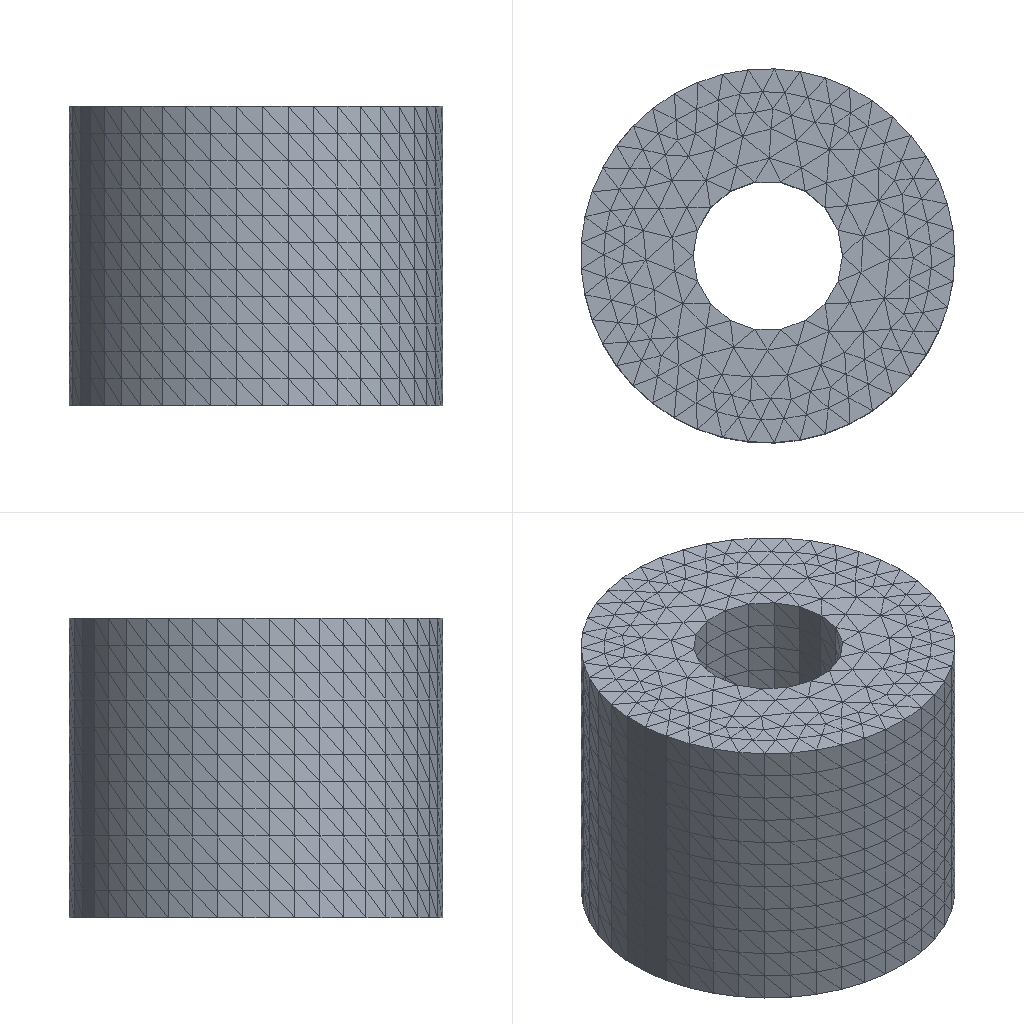Simulation study | abaqus
Notes in the study folder:
10 truncated cone proxy hollow cyl
job_status=None
Umax_mm=0.000227654
S_Mises_max_MPa=1.64312
Set-up summary:
category,name,step,type,value,unit,region
solver,abaqus,,Abaqus/CAE 2024
units,mm-N-s-tonne (MPa),,inferred,E=210000 density=7.85e-09
analysis,Step-1,,static,time_period=1
mesh,nodes,,,14772
mesh,elements,,,9526
element_type,C3D10,,,9526
material,Steel,,E,210000
material,Steel,,nu,0.3
material,Steel,,density,7.85e-09
section,Steel,,solid section,,,_PickedSet2
load,Load,Step-1,pressure,1.2,,TOP
bc,BC,Step-1,encastre,[dofs=ENCASTRE],,FIXED
Abaqus input file, long lists of numbers shortened:
*Heading
** Job name: deck Model name: M10
** Generated by: Abaqus/CAE 2024
*Preprint, echo=NO, model=NO, history=NO, contact=NO
**
** PARTS
**
*Part, name=P
*Node
      1,          10.,           0.,          40.
      2,          10.,           0.,           0.
** (14770 more lines like these left out)
*Element, type=C3D10
   1,  1023,  1024,  1025,  1026,  2115,  2114,  2113,  2117,  2116,  2118
   2,  1023,  1027,  1028,  1029,  2121,  2120,  2119,  2123,  2122,  2124
** (9524 more lines like these left out)
*Nset, nset=_PickedSet2, internal, generate
     1,  14772,      1
*Elset, elset=_PickedSet2, internal, generate
    1,  9526,     1
** Section: Sec
*Solid Section, elset=_PickedSet2, material=Steel
,
*End Part
**
**
** ASSEMBLY
**
*Assembly, name=Assembly
**
*Instance, name=I, part=P
*End Instance
**
*Nset, nset=FIXED, instance=I
     2,     3,    22,    23,    24,    25,    26,    27,    28,    29,    30,    31,    32,    33,    34,    35
    36,    37,    38,    39,    40,    41,    42,    43,    44,    45,    46,    47,    48,    49,    50,    51
** (44 more lines like these left out)
*Elset, elset=FIXED, instance=I
  397,  435,  834,  852,  935, 1189, 1262, 1283, 1497, 1519, 1644, 1650, 1651, 1664, 1691, 1733
 1764, 1777, 1793, 2028, 2155, 2199, 2355, 2479, 2495, 2592, 2595, 2600, 2697, 2707, 2717, 2718
** (19 more lines like these left out)
*Elset, elset=_TOP_S3, internal, instance=I
  138,  312,  317,  673,  826,  972, 1037, 1170, 1242, 1408, 1609, 1639, 1640, 1653, 1708, 1714
 1724, 1747, 1752, 1756, 1790, 1802, 1835, 1840, 1847, 1889, 1903, 1912, 1969, 1975, 1986, 1991
** (15 more lines like these left out)
*Elset, elset=_TOP_S2, internal, instance=I
 1077, 1711, 1721, 4206, 4228, 4253, 4294, 4345, 4453, 4462, 4587, 4737, 4883, 4947, 4988, 5093
 5241, 8839
*Elset, elset=_TOP_S4, internal, instance=I
 1252, 1649, 1659, 1859, 1869, 1927, 1945, 1955, 1978, 2044, 4320, 4657, 4677, 4723, 4767, 4779
 4853, 4965, 4983, 5040, 5051, 5115, 5176, 5334, 5440, 5849, 5858, 6696, 6999, 7060, 9339
*Elset, elset=_TOP_S1, internal, instance=I
 1952, 4083, 4127, 4310, 4348, 4410, 8876, 8928
*Surface, type=ELEMENT, name=TOP
_TOP_S3, S3
_TOP_S2, S2
_TOP_S4, S4
_TOP_S1, S1
*End Assembly
**
** MATERIALS
**
*Material, name=Steel
*Density
 7.85e-09,
*Elastic
210000., 0.3
** ----------------------------------------------------------------
**
** STEP: Step-1
**
*Step, name=Step-1, nlgeom=NO
*Static
1., 1., 1e-05, 1.
**
** BOUNDARY CONDITIONS
**
** Name: BC Type: Symmetry/Antisymmetry/Encastre
*Boundary
FIXED, ENCASTRE
**
** LOADS
**
** Name: Load   Type: Pressure
*Dsload
TOP, P, 1.2
**
** OUTPUT REQUESTS
**
*Restart, write, frequency=0
**
** FIELD OUTPUT: F-Output-1
**
*Output, field, variable=PRESELECT
**
** HISTORY OUTPUT: H-Output-1
**
*Output, history, variable=PRESELECT
*End Step
Results summary:
result,odb.job_status,,,JOB_STATUS_COMPLETED_SUCCESSFULLY,"consistent, unstated (Abaqus has no unit system)"
result,steps[0].procedure,Step-1,,*STATIC,"consistent, unstated (Abaqus has no unit system)"
result,steps[0].time_period,Step-1,,1,"consistent, unstated (Abaqus has no unit system)"
result,steps[0].n_frames,Step-1,,2,"consistent, unstated (Abaqus has no unit system)"
result,steps[0].last_frame.id,Step-1,,1,"consistent, unstated (Abaqus has no unit system)"
result,steps[0].last_frame.value,Step-1,,1,"consistent, unstated (Abaqus has no unit system)"
result,steps[0].last_frame.description,Step-1,,Increment      1: Step Time =    1.000,"consistent, unstated (Abaqus has no unit system)"
result,steps[0].completed,Step-1,,True,"consistent, unstated (Abaqus has no unit system)"
result,steps[0].max_U_magnitude,Step-1,,0.0002277,"consistent, unstated (Abaqus has no unit system)"
result,steps[0].max_S_mises,Step-1,,1.643,"consistent, unstated (Abaqus has no unit system)"
result,steps[0].RF_sum[1],Step-1,,1.09971e-05,"consistent, unstated (Abaqus has no unit system)"
result,steps[0].RF_sum[2],Step-1,,-8.9407e-07,"consistent, unstated (Abaqus has no unit system)"
result,steps[0].RF_sum[3],Step-1,,1979.21,"consistent, unstated (Abaqus has no unit system)"
result,steps[1].procedure,Step-1,,*STATIC,"consistent, unstated (Abaqus has no unit system)"
result,steps[1].time_period,Step-1,,1,"consistent, unstated (Abaqus has no unit system)"
result,steps[1].n_frames,Step-1,,2,"consistent, unstated (Abaqus has no unit system)"
result,steps[1].last_frame.id,Step-1,,1,"consistent, unstated (Abaqus has no unit system)"
result,steps[1].last_frame.value,Step-1,,1,"consistent, unstated (Abaqus has no unit system)"
result,steps[1].last_frame.description,Step-1,,Increment      1: Step Time =    1.000,"consistent, unstated (Abaqus has no unit system)"
result,steps[1].completed,Step-1,,True,"consistent, unstated (Abaqus has no unit system)"
result,steps[1].max_U_magnitude,Step-1,,0.0002277,"consistent, unstated (Abaqus has no unit system)"
result,steps[1].max_S_mises,Step-1,,1.643,"consistent, unstated (Abaqus has no unit system)"
result,steps[1].RF_sum[1],Step-1,,1.09971e-05,"consistent, unstated (Abaqus has no unit system)"
result,steps[1].RF_sum[2],Step-1,,-8.9407e-07,"consistent, unstated (Abaqus has no unit system)"
result,steps[1].RF_sum[3],Step-1,,1979.21,"consistent, unstated (Abaqus has no unit system)"